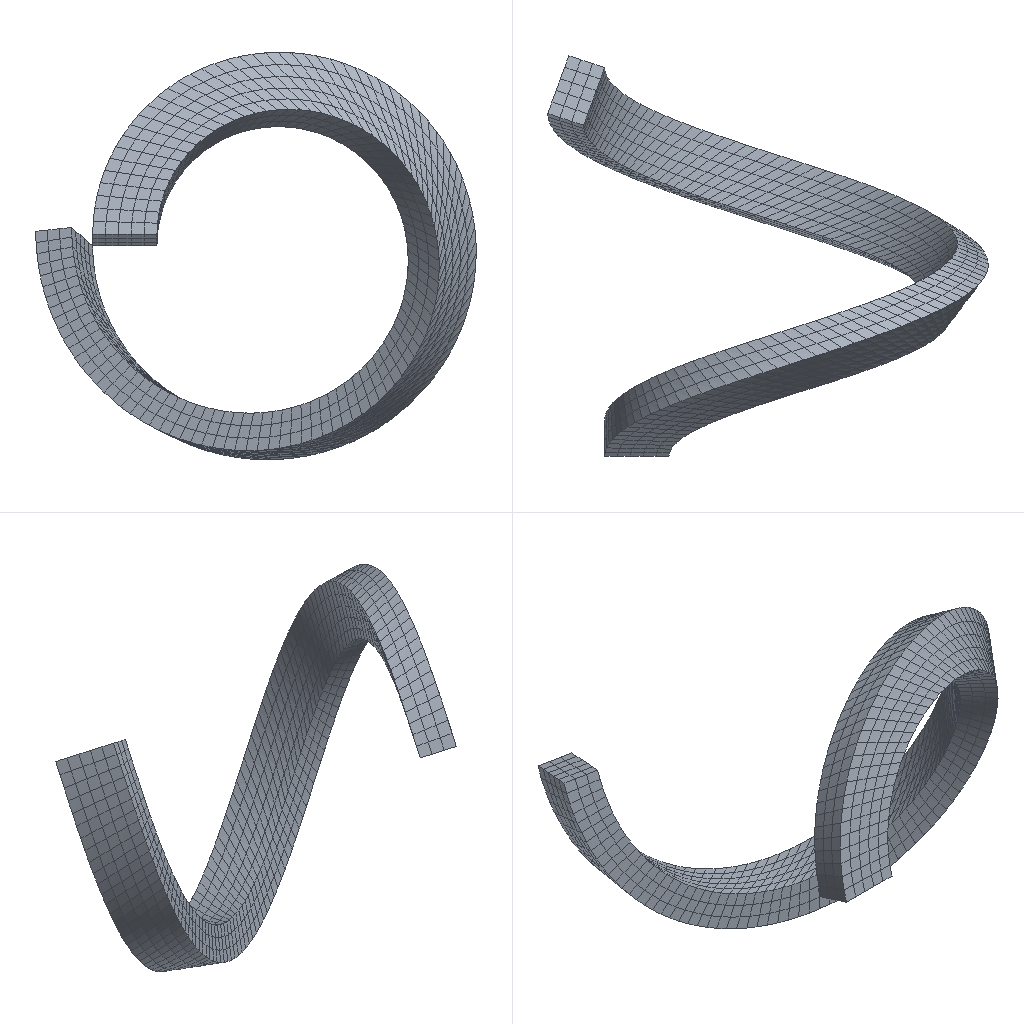Simulation study | abaqus
Set-up summary:
category,name,step,type,value,unit,region
solver,abaqus
solver,version,,,Abaqus/Explicit 2020
units,not stated in the deck,,not stated
analysis,deck,,transient,transient
load_step,Step-1,Step-1,transient,nlgeom=True
load_step,Step-2,Step-2,transient,nlgeom=True
contact,interactions,,,general=1 pairs=0 ties=1
load_step,requested,,,2
mesh,nodes,,,7532
mesh,elements,,,6440
element_type,R3D4,,rigid,5000
element_type,C3D8R,,solid,1440
load,load commands in deck,,count,3
bc,support commands in deck,,count,14
material,MATERIAL-1,,in results
check,setup vs results,,match,"per instance, exact: element labels, types and connectivity; labels of the nodes the elements use; coordinates not compared"
Abaqus input file, long lists of numbers shortened:
*Heading
** Job name: Job-1 Model name: Model-1
** Generated by: Abaqus/CAE 2020
*Preprint, echo=NO, model=NO, history=NO, contact=NO
**
** PARTS
**
*Part, name=rig
*Node
      1,          0.5,           0.,           0.
      2,   0.49,           0.,           0.
** (2599 more lines like these left out)
*Element, type=R3D4
   1,    1,    2,   53,   52
   2,    2,    3,   54,   53
** (2498 more lines like these left out)
*Node
   2602,         0.25,        -0.25,           0.
*Nset, nset=rig-RefPt_, internal
2602,
*Elset, elset=rig, generate
    1,  2500,     1
*End Part
**
*Part, name=xianwei
*Node
      1,  -0.1805,  0.3101, -0.003218
      2, -0.1841,  0.3003, -8.66764676e-05
** (2326 more lines like these left out)
*Element, type=C3D8R
   1,   25,   26,   32,   31,    1,    2,    8,    7
   2,   26,   27,   33,   32,    2,    3,    9,    8
** (1438 more lines like these left out)
*Nset, nset=Set-1, generate
    1,  2328,     1
*Elset, elset=Set-1, generate
    1,  1440,     1
** Section: Section-1
*Solid Section, elset=Set-1, material=Material-1
,
*End Part
**
**
** ASSEMBLY
**
*Assembly, name=Assembly
**
*Instance, name=xianwei-1, part=xianwei
*End Instance
**
*Instance, name=rig-1, part=rig
   -0.2727,    -0.03178,     0.2398
   -0.2727,    -0.03178,     0.2398, -0.85, 0.5456, 0.8171,         120.
*End Instance
**
*Instance, name=rig-1-lin-2-1, part=rig
   -0.2727,     0.3132,     0.2398
   -0.2727,     0.3132,     0.2398, -0.85, 0.8906, 0.8171,         120.
*End Instance
**
*Nset, nset=Set-1, instance=xianwei-1
  1, 19
*Nset, nset=Set-2, instance=xianwei-1
 2305, 2310
*Nset, nset=Set-3, instance=rig-1
 2602,
*Nset, nset=Set-4, instance=rig-1-lin-2-1
 2602,
*Nset, nset=s_Set-5, instance=xianwei-1, generate
 2305,  2310,     1
*Elset, elset=s_Set-5, instance=xianwei-1, generate
 1426,  1430,     1
*Elset, elset=_m_Surf-1_SPOS, internal, instance=rig-1, generate
    1,  2500,     1
*Surface, type=ELEMENT, name=m_Surf-1
_m_Surf-1_SPOS, SPOS
*Surface, type=NODE, name=s_Set-5_CNS_, internal
s_Set-5, 1.
*Rigid Body, ref node=rig-1.rig-RefPt_, elset=rig-1.rig
*Rigid Body, ref node=rig-1-lin-2-1.rig-RefPt_, elset=rig-1-lin-2-1.rig
** Constraint: Constraint-1
*Tie, name=Constraint-1, adjust=yes
s_Set-5_CNS_, m_Surf-1
*End Assembly
*Amplitude, name=Amp-1
             0.,              0.,           0.001,              1.
**
** MATERIALS
**
*Material, name=Material-1
*Density
 3.05e-09,
*Elastic
109000., 0.28
**
** INTERACTION PROPERTIES
**
*Surface Interaction, name=IntProp-1
*Friction
 0.15,
*Surface Behavior, pressure-overclosure=HARD
**
** INTERACTIONS
**
** Interaction: Int-1
*Contact, op=NEW
*Contact Inclusions, ALL EXTERIOR
*Contact Property Assignment
 ,  , IntProp-1
** ----------------------------------------------------------------
**
** STEP: Step-1
**
*Step, name=Step-1, nlgeom=YES
*Dynamic, Explicit
, 0.001
*Bulk Viscosity
0.06, 1.2
** Mass Scaling: Semi-Automatic
**               Whole Model
*Fixed Mass Scaling, factor=500.
**
** BOUNDARY CONDITIONS
**
** Name: [REDACTED]
*Boundary, amplitude=Amp-1
Set-4, 1, 1
Set-4, 2, 2, -0.15
Set-4, 3, 3
Set-4, 4, 4
Set-4, 5, 5
Set-4, 6, 6
** Name: [REDACTED]
*Boundary, amplitude=Amp-1
Set-3, 1, 1
Set-3, 2, 2, 0.15
Set-3, 3, 3
Set-3, 4, 4
Set-3, 5, 5
Set-3, 6, 6
**
** OUTPUT REQUESTS
**
*Restart, write, number interval=1, time marks=NO
**
** FIELD OUTPUT: F-Output-1
**
*Output, field
*Node Output
CF, RF, RM, RT, U, V
*Element Output, directions=YES
E, LE, MISES, MISESMAX, MISESONLY, PE, PEEQ, PEEQMAX, PEEQT, PEMAG, PRESSONLY, S, SEQUT, SSAVG, YIELDPOT
*Contact Output
CDISP, CSTRESS
**
** HISTORY OUTPUT: H-Output-1
**
*Output, history, variable=PRESELECT, frequency=1
*End Step
** ----------------------------------------------------------------
**
** STEP: Step-2
**
*Step, name=Step-2, nlgeom=YES
*Dynamic, Explicit
, 0.001
*Bulk Viscosity
0.06, 1.2
** Mass Scaling: Semi-Automatic
**               Whole Model
*Fixed Mass Scaling, factor=500.
**
** BOUNDARY CONDITIONS
**
** Name: [REDACTED]
*Boundary, amplitude=Amp-1
Set-4, 2, 2, 0.35
** Name: [REDACTED]
*Boundary, amplitude=Amp-1
Set-3, 2, 2
**
** OUTPUT REQUESTS
**
*Restart, write, number interval=1, time marks=NO
**
** FIELD OUTPUT: F-Output-1
**
*Output, field
*Node Output
CF, RF, RM, RT, U, V
*Element Output, directions=YES
E, LE, MISES, MISESMAX, MISESONLY, PE, PEEQ, PEEQMAX, PEEQT, PEMAG, PRESSONLY, S, SEQUT, SSAVG, YIELDPOT
*Contact Output
CDISP, CSTRESS
**
** HISTORY OUTPUT: H-Output-1
**
*Output, history, variable=PRESELECT, frequency=1
*End Step
Results summary:
result,step,Step-1,completed,increments=63517 time=0.001/0.001
result,step,Step-2,completed,increments=65682 time=0.001/0.001
result,analysis,,,transient
result,last_loadstep,,,2
result,analysis steps,,count,2
result,primary field,,,U
result,reaction total,,FX,0.0,model units
result,reaction total,,FY,0.0,model units
result,reaction total,,FZ,0.0,model units